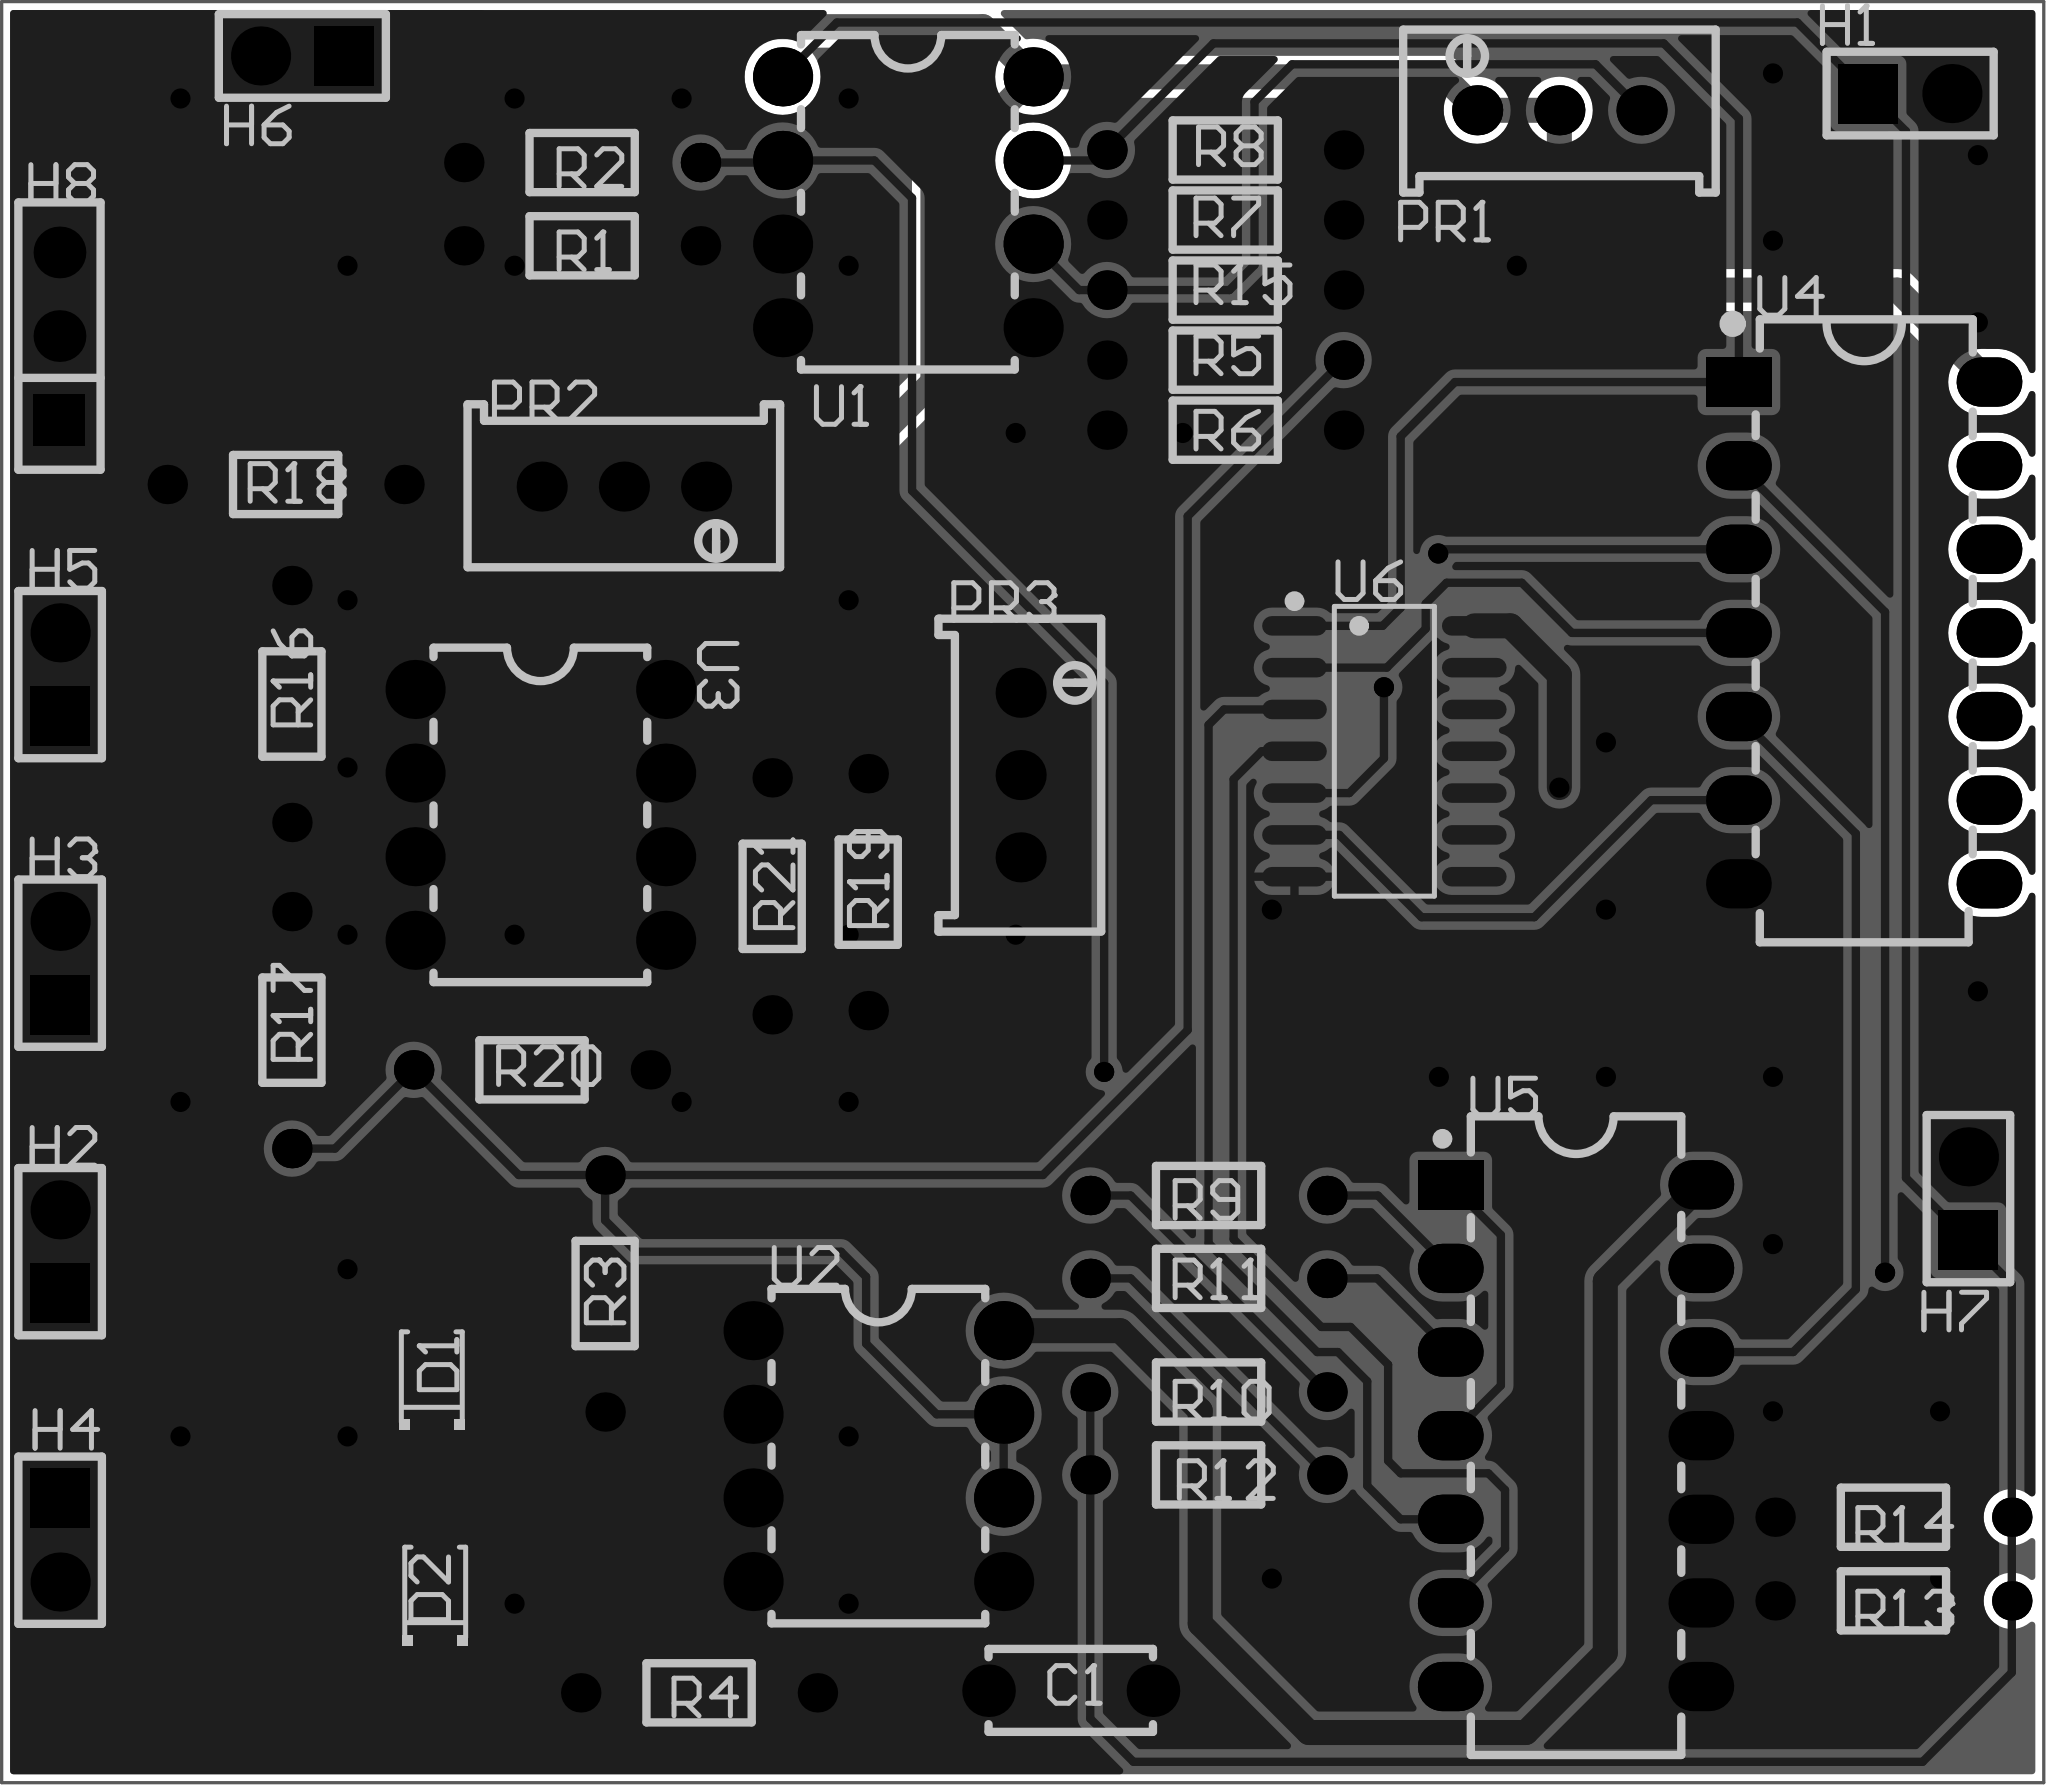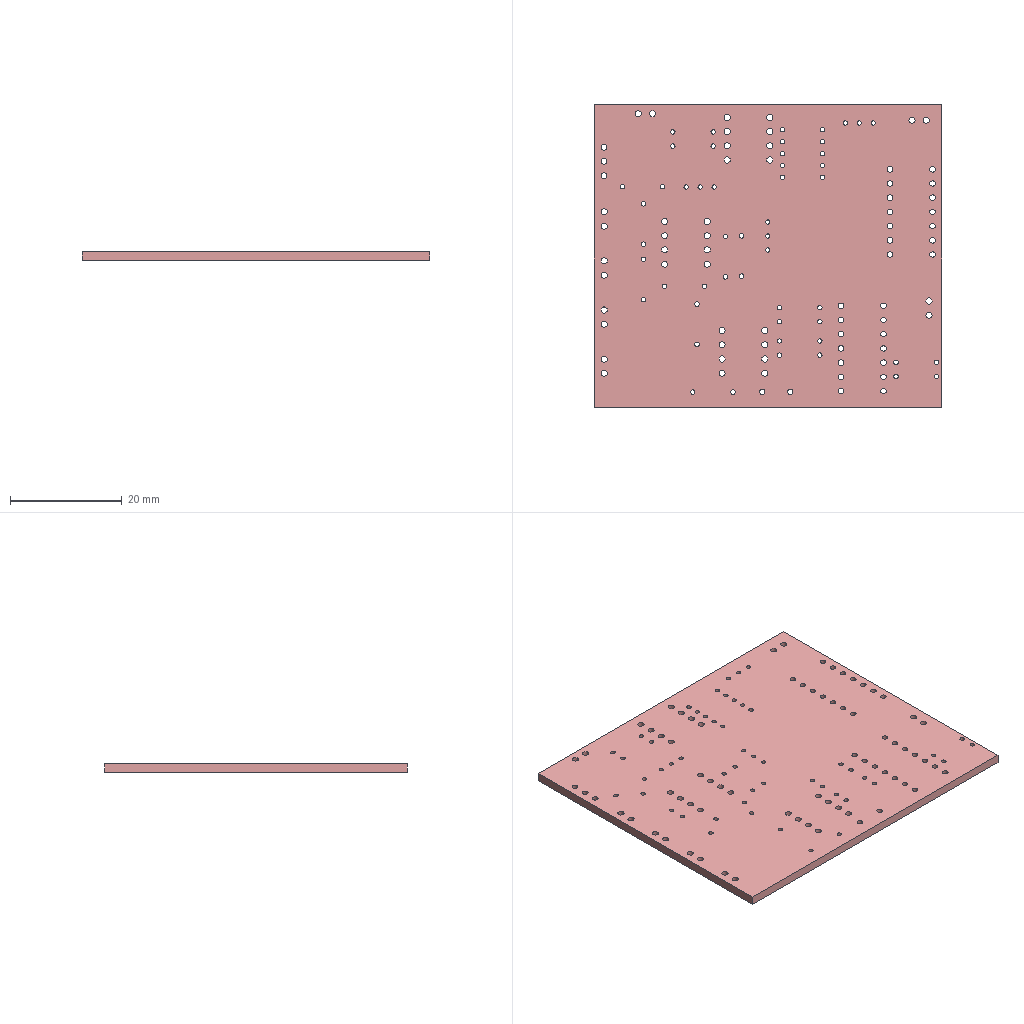Circuit board layout | Altium Designer | box 62.1 x 54.1 x 1.6 mm
Layer stack:
# Altium Designer layer stack of  (unit mm; dielectric type: 0 none, 1 core, 2 prepreg, 3 surface material)
index,name,kind,layer,copper_thickness_mm,dielectric_type,dielectric_thickness_mm,dielectric_material,dielectric_constant
0,Top Paste Mask Layer,other,,,,,,
1,Top Silkscreen Layer,other,,,,,,
2,Top Solder Mask Layer,dielectric,,,3,0.01,,3.3
3,Top Layer,copper,Top Layer,0.035,,,,
4,Dielectric1,dielectric,,,3,1.51,FR4,4.5
5,Bottom Layer,copper,Bottom Layer,0.035,,,,
6,Bottom Solder Mask Layer,dielectric,,,3,0.01,,3.3
7,Bottom Silkscreen Layer,other,,,,,,
8,Bottom Paste Mask Layer,other,,,,,,
# drill layer pairs: low layer,high layer
drill_pair,Top Layer,Bottom Layer
Part placement:
Designator,Comment,Layer,Footprint,Center-X(mm),Center-Y(mm),Rotation
D1,1N4148W,TopLayer,SOD-123F_L2.7-W1.6-LS3.8-RD,92.329,93.98,90
D2,1N4148W,TopLayer,SOD-123F_L2.7-W1.6-LS3.8-RD,92.433,87.439,90
H1,,TopLayer,HDR-TH_2P-P2.54-V-M-1,137.287,132.969,0
H2,,TopLayer,HDR-TH_2P-P2.54-V-M-1,81.026,97.791,90
H3,,TopLayer,HDR-TH_2P-P2.54-V-M-1,81.026,106.555,90
H4,,TopLayer,HDR-TH_2P-P2.54-V-M-1,81.026,89.027,270
H5,,TopLayer,HDR-TH_2P-P2.54-V-M-1,81.026,115.319,90
H6,,TopLayer,HDR-TH_2P-P2.54-V-M-1,88.392,134.112,180
H7,,TopLayer,HDR-TH_2P-P2.54-V-M-1,139.06,99.402,90
H8,,TopLayer,HDR-TH_3P-P2.54-V-F,81.006,125.603,90
PR1,51kΩ,TopLayer,R_3296,126.619,132.461,0
PR2,51kΩ,TopLayer,R_3296,98.171,121.031,180
PR3,51kΩ,TopLayer,R_3296,110.236,112.268,270
U1,LM358AP,TopLayer,PDIP-8_L10.2-W6.5-P2.54-LS7.6-BL,106.807,129.667,270
U2,LM358AN/NOPB,TopLayer,PDIP-8_L10.2-W6.5-P2.54-LS7.6-BL,105.91,91.581,270
U3,LM358AN/NOPB,TopLayer,PDIP-8_L10.2-W6.5-P2.54-LS7.6-BL,95.631,111.058,270
U4,CD40106BD,TopLayer,DIP-14_L19.1-W6.4-P2.54-LS7.6-BL,135.89,116.586,270
U5,SN74LV4066AN,TopLayer,PDIP-14_L19.3-W6.4-P2.54-LS7.9-BL-1,127.127,92.202,270
U6,HEF4081BT118,TopLayer,SO-14_L8.9-W3.9-P1.27-LS6.0-BL,121.298,112.991,270
C1,22uF,TopLayer,CAP-TH_L5.0-W2.5-P5.00-D1.0,111.76,84.455,180
R1,10K,TopLayer,Res_1/8W,96.901,128.345,0
R2,10K,TopLayer,Res_1/8W,96.901,130.873,0
R3,1K,TopLayer,Res_1/8W,97.6,96.52,90
R4,10K,TopLayer,Res_1/8W,100.457,84.391,0
R5,1K,TopLayer,Res_1/8W,116.459,124.873,180
R6,100K,TopLayer,Res_1/8W,116.459,122.745,0
R7,82K,TopLayer,Res_1/8W,116.459,129.128,0
R8,5.1K,TopLayer,Res_1/8W,116.459,131.255,180
R9,45K,TopLayer,Res_1/8W,115.952,99.497,180
R10,5.1K,TopLayer,Res_1/8W,115.952,93.528,180
R11,39K,TopLayer,Res_1/8W,115.952,96.979,180
R12,1K,TopLayer,Res_1/8W,115.952,91.01,180
R13,20K,TopLayer,Res_1/8W,136.779,87.185,0
R14,9.5K,TopLayer,Res_1/8W,136.779,89.725,0
R15,2K,TopLayer,Res_1/8W,116.459,127,180
R16,75K,TopLayer,Res_1/8W,88.075,114.427,90
R17,1K,TopLayer,Res_1/8W,88.075,104.521,90
R18,2K,TopLayer,Res_1/8W,87.884,121.094,0
R19,2K,TopLayer,Res_1/8W,105.601,108.712,90
R20,1K,TopLayer,Res_1/8W,95.377,103.314,0
R21,75K,TopLayer,Res_1/8W,102.68,108.585,90
Pad and via stacks:
# Altium Designer via and pad stacks of  (unit mm). Each distinct definition once, with the count of objects using it.
# via: kind,start_layer,end_layer,hole_mm,diameter_mm,mode(0 simple;1 top-mid-bottom;2 full stack),diameter_per_layer,count,example_net
# pad: kind,layer,hole_mm,hole_type(0 round;1 square;2 slot),plating,top_size,top_shape(1 round;2 rect;3 octagon;9 rounded rect),mid_size,bottom_size,mode,footprint,size_per_layer,count,example
pad,Top Layer,0,0,plated,1.1x1,2,1.1x1,1.1x1,0,SOD-123F_L2.7-W1.6-LS3.8-RD,,4,D1.2
pad,Top Layer,0,0,plated,0.595x1.968,1,0.595x1.968,0.595x1.968,0,SO-14_L8.9-W3.9-P1.27-LS6.0-BL,,14,U6.1
pad,Multi-Layer,1.1,0,plated,1.8x1.8,1,1.8x1.8,1.8x1.8,0,HDR-TH_2P-P2.54-V-M-1,,7,H1.2
pad,Multi-Layer,1.1,0,plated,1.8x1.8,2,1.8x1.8,1.8x1.8,0,HDR-TH_2P-P2.54-V-M-1,,7,H1.1
pad,Multi-Layer,1.02,0,plated,1.575x1.575,1,1.575x1.575,1.575x1.575,0,HDR-TH_3P-P2.54-V-F,,2,H8.3
pad,Multi-Layer,1.02,0,plated,1.575x1.575,2,1.575x1.575,1.575x1.575,0,HDR-TH_3P-P2.54-V-F,,1,H8.1
pad,Multi-Layer,0.762,0,plated,1.524x1.524,1,1.524x1.524,1.524x1.524,0,R_3296,,9,PR1.2
pad,Multi-Layer,1.1,0,plated,1.8x1.8,1,1.8x1.8,1.8x1.8,0,PDIP-8_L10.2-W6.5-P2.54-LS7.6-BL,,24,U1.1
pad,Multi-Layer,1,0,plated,2x1.5,1,2x1.5,2x1.5,0,DIP-14_L19.1-W6.4-P2.54-LS7.6-BL,,13,U4.8
pad,Multi-Layer,1,0,plated,2x1.5,2,2x1.5,2x1.5,0,DIP-14_L19.1-W6.4-P2.54-LS7.6-BL,,1,U4.1
pad,Multi-Layer,1,0,plated,2x1.5,2,2x1.5,2x1.5,0,PDIP-14_L19.3-W6.4-P2.54-LS7.9-BL-1,,1,U5.1
pad,Multi-Layer,1,0,plated,2x1.5,1,2x1.5,2x1.5,0,PDIP-14_L19.3-W6.4-P2.54-LS7.9-BL-1,,13,U5.2
pad,Multi-Layer,1,0,plated,1.6x1.6,1,1.6x1.6,1.6x1.6,0,CAP-TH_L5.0-W2.5-P5.00-D1.0,,2,C1.1
pad,Multi-Layer,0.8001,0,plated,1.199x1.199,1,1.199x1.199,1.199x1.199,0,Res_1/8W,,42,R1.1
via,Top Layer,Bottom Layer,0.3048,0.61,0,,47,OUT1
Copper pours:
name,layer,net,type(0 solid;1 hatched;2 none)
Bottom Layer-GND,Bottom Layer,GND,0
Top Layer-GND,Top Layer,GND,0
Design rules, without the lines most boards share:
# Altium Designer design rules of  (exported by Altium Designer, unit mm)
# columns: name | kind | enabled | priority | scope1 | scope2 | descriptor | typed fields (field=value)
creepage | 65 | enabled | 1 | All | All | Creepage Distance Constraint =(0mil) (All),(All) |